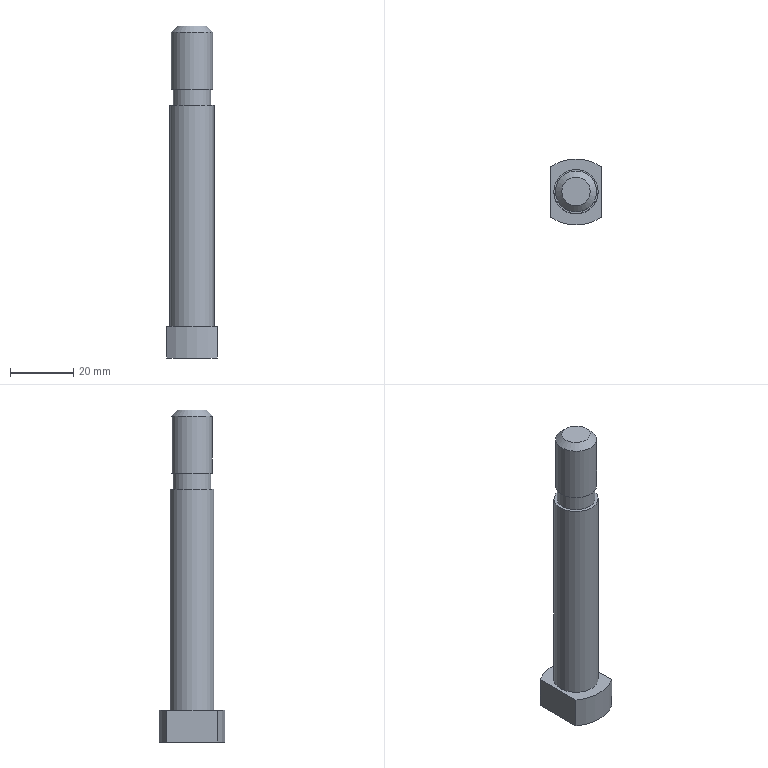Part | NX | features EXTRUDE 4, DATUM_CSYS 2, CHAMFER 1, SKETCH 1 | 1 solid | 13 faces | box 16 x 21.022 x 105 mm | volume 17029 mm3 | plane 7 | cylinder 5 | cone 1 | commonest cylinder face diameters 28 x2 12 x1 13 x1 14 x1
STEP:
#1=CARTESIAN_POINT('',(-8.,-8.,0.));
#2=VERTEX_POINT('',#1);
#3=CARTESIAN_POINT('',(-8.,8.,0.));
#4=VERTEX_POINT('',#3);
#5=CARTESIAN_POINT('',(-8.,-8.,0.));
#6=DIRECTION('',(0.,1.,0.));
#7=VECTOR('',#6,1000.);
#8=LINE('',#5,#7);
#9=EDGE_CURVE('',#2,#4,#8,.T.);
#10=ORIENTED_EDGE('',*,*,#9,.F.);
#11=CARTESIAN_POINT('',(-8.,-8.,10.));
#12=VERTEX_POINT('',#11);
#13=CARTESIAN_POINT('',(-8.,-8.,10.));
#14=DIRECTION('',(0.,0.,-1.));
#15=VECTOR('',#14,1000.);
#16=LINE('',#13,#15);
#17=EDGE_CURVE('',#12,#2,#16,.T.);
#18=ORIENTED_EDGE('',*,*,#17,.F.);
#19=CARTESIAN_POINT('',(-8.,8.,10.));
#20=VERTEX_POINT('',#19);
#21=CARTESIAN_POINT('',(-8.,-8.,10.));
#22=DIRECTION('',(0.,1.,0.));
#23=VECTOR('',#22,1000.);
#24=LINE('',#21,#23);
#25=EDGE_CURVE('',#12,#20,#24,.T.);
#26=ORIENTED_EDGE('',*,*,#25,.T.);
#27=CARTESIAN_POINT('',(-8.,8.,10.));
#28=DIRECTION('',(0.,0.,-1.));
#29=VECTOR('',#28,1000.);
#30=LINE('',#27,#29);
#31=EDGE_CURVE('',#20,#4,#30,.T.);
#32=ORIENTED_EDGE('',*,*,#31,.T.);
#33=EDGE_LOOP('',(#10,#18,#26,#32));
#34=FACE_BOUND('',#33,.T.);
#35=CARTESIAN_POINT('',(-8.,-8.,10.));
#36=DIRECTION('',(-1.,0.,0.));
#37=DIRECTION('',(0.,-1.,0.));
#38=AXIS2_PLACEMENT_3D('',#35,#36,#37);
#39=PLANE('',#38);
#40=ADVANCED_FACE('',(#34),#39,.T.);
#41=CARTESIAN_POINT('',(8.,8.,0.));
#42=VERTEX_POINT('',#41);
#43=CARTESIAN_POINT('',(0.,-3.489,0.));
#44=DIRECTION('',(0.,0.,-1.));
#45=DIRECTION('',(1.,0.,0.));
#46=AXIS2_PLACEMENT_3D('',#43,#44,#45);
#47=CIRCLE('',#46,14.);
#48=EDGE_CURVE('',#4,#42,#47,.T.);
#49=ORIENTED_EDGE('',*,*,#48,.F.);
#50=ORIENTED_EDGE('',*,*,#31,.F.);
#51=CARTESIAN_POINT('',(8.,8.,10.));
#52=VERTEX_POINT('',#51);
#53=CARTESIAN_POINT('',(0.,-3.489,10.));
#54=DIRECTION('',(0.,0.,-1.));
#55=DIRECTION('',(1.,0.,0.));
#56=AXIS2_PLACEMENT_3D('',#53,#54,#55);
#57=CIRCLE('',#56,14.);
#58=EDGE_CURVE('',#20,#52,#57,.T.);
#59=ORIENTED_EDGE('',*,*,#58,.T.);
#60=CARTESIAN_POINT('',(8.,8.,10.));
#61=DIRECTION('',(0.,0.,-1.));
#62=VECTOR('',#61,1000.);
#63=LINE('',#60,#62);
#64=EDGE_CURVE('',#52,#42,#63,.T.);
#65=ORIENTED_EDGE('',*,*,#64,.T.);
#66=EDGE_LOOP('',(#49,#50,#59,#65));
#67=FACE_BOUND('',#66,.T.);
#68=CARTESIAN_POINT('',(0.,-3.489,10.));
#69=DIRECTION('',(0.,0.,-1.));
#70=DIRECTION('',(-1.,0.,0.));
#71=AXIS2_PLACEMENT_3D('',#68,#69,#70);
#72=CYLINDRICAL_SURFACE('',#71,14.);
#73=ADVANCED_FACE('',(#67),#72,.T.);
#74=CARTESIAN_POINT('',(8.,-8.,0.));
#75=VERTEX_POINT('',#74);
#76=CARTESIAN_POINT('',(8.,8.,0.));
#77=DIRECTION('',(0.,-1.,0.));
#78=VECTOR('',#77,1000.);
#79=LINE('',#76,#78);
#80=EDGE_CURVE('',#42,#75,#79,.T.);
#81=ORIENTED_EDGE('',*,*,#80,.F.);
#82=ORIENTED_EDGE('',*,*,#64,.F.);
#83=CARTESIAN_POINT('',(8.,-8.,10.));
#84=VERTEX_POINT('',#83);
#85=CARTESIAN_POINT('',(8.,8.,10.));
#86=DIRECTION('',(0.,-1.,0.));
#87=VECTOR('',#86,1000.);
#88=LINE('',#85,#87);
#89=EDGE_CURVE('',#52,#84,#88,.T.);
#90=ORIENTED_EDGE('',*,*,#89,.T.);
#91=CARTESIAN_POINT('',(8.,-8.,10.));
#92=DIRECTION('',(0.,0.,-1.));
#93=VECTOR('',#92,1000.);
#94=LINE('',#91,#93);
#95=EDGE_CURVE('',#84,#75,#94,.T.);
#96=ORIENTED_EDGE('',*,*,#95,.T.);
#97=EDGE_LOOP('',(#81,#82,#90,#96));
#98=FACE_BOUND('',#97,.T.);
#99=CARTESIAN_POINT('',(8.,8.,10.));
#100=DIRECTION('',(1.,0.,0.));
#101=DIRECTION('',(0.,1.,0.));
#102=AXIS2_PLACEMENT_3D('',#99,#100,#101);
#103=PLANE('',#102);
#104=ADVANCED_FACE('',(#98),#103,.T.);
#105=CARTESIAN_POINT('',(0.,3.489,0.));
#106=DIRECTION('',(0.,0.,-1.));
#107=DIRECTION('',(1.,0.,0.));
#108=AXIS2_PLACEMENT_3D('',#105,#106,#107);
#109=CIRCLE('',#108,14.);
#110=EDGE_CURVE('',#75,#2,#109,.T.);
#111=ORIENTED_EDGE('',*,*,#110,.F.);
#112=ORIENTED_EDGE('',*,*,#95,.F.);
#113=CARTESIAN_POINT('',(0.,3.489,10.));
#114=DIRECTION('',(0.,0.,-1.));
#115=DIRECTION('',(1.,0.,0.));
#116=AXIS2_PLACEMENT_3D('',#113,#114,#115);
#117=CIRCLE('',#116,14.);
#118=EDGE_CURVE('',#84,#12,#117,.T.);
#119=ORIENTED_EDGE('',*,*,#118,.T.);
#120=ORIENTED_EDGE('',*,*,#17,.T.);
#121=EDGE_LOOP('',(#111,#112,#119,#120));
#122=FACE_BOUND('',#121,.T.);
#123=CARTESIAN_POINT('',(0.,3.489,10.));
#124=DIRECTION('',(0.,0.,-1.));
#125=DIRECTION('',(-1.,0.,0.));
#126=AXIS2_PLACEMENT_3D('',#123,#124,#125);
#127=CYLINDRICAL_SURFACE('',#126,14.);
#128=ADVANCED_FACE('',(#122),#127,.T.);
#129=CARTESIAN_POINT('',(7.,0.,10.));
#130=VERTEX_POINT('',#129);
#131=CARTESIAN_POINT('',(0.,0.,10.));
#132=DIRECTION('',(0.,0.,1.));
#133=DIRECTION('',(1.,0.,0.));
#134=AXIS2_PLACEMENT_3D('',#131,#132,#133);
#135=CIRCLE('',#134,7.);
#136=EDGE_CURVE('',#130,#130,#135,.T.);
#137=ORIENTED_EDGE('',*,*,#136,.F.);
#138=EDGE_LOOP('',(#137));
#139=FACE_BOUND('',#138,.T.);
#140=ORIENTED_EDGE('',*,*,#25,.F.);
#141=ORIENTED_EDGE('',*,*,#118,.F.);
#142=ORIENTED_EDGE('',*,*,#89,.F.);
#143=ORIENTED_EDGE('',*,*,#58,.F.);
#144=EDGE_LOOP('',(#140,#141,#142,#143));
#145=FACE_BOUND('',#144,.T.);
#146=CARTESIAN_POINT('',(0.,-3.489,10.));
#147=DIRECTION('',(0.,0.,-1.));
#148=DIRECTION('',(-1.,0.,0.));
#149=AXIS2_PLACEMENT_3D('',#146,#147,#148);
#150=PLANE('',#149);
#151=ADVANCED_FACE('',(#139,#145),#150,.F.);
#152=ORIENTED_EDGE('',*,*,#9,.T.);
#153=ORIENTED_EDGE('',*,*,#48,.T.);
#154=ORIENTED_EDGE('',*,*,#80,.T.);
#155=ORIENTED_EDGE('',*,*,#110,.T.);
#156=EDGE_LOOP('',(#152,#153,#154,#155));
#157=FACE_BOUND('',#156,.T.);
#158=CARTESIAN_POINT('',(0.,-3.489,0.));
#159=DIRECTION('',(0.,0.,-1.));
#160=DIRECTION('',(-1.,0.,0.));
#161=AXIS2_PLACEMENT_3D('',#158,#159,#160);
#162=PLANE('',#161);
#163=ADVANCED_FACE('',(#157),#162,.T.);
#164=CARTESIAN_POINT('',(7.,0.,80.));
#165=VERTEX_POINT('',#164);
#166=CARTESIAN_POINT('',(0.,0.,80.));
#167=DIRECTION('',(0.,0.,1.));
#168=DIRECTION('',(1.,0.,0.));
#169=AXIS2_PLACEMENT_3D('',#166,#167,#168);
#170=CIRCLE('',#169,7.);
#171=EDGE_CURVE('',#165,#165,#170,.T.);
#172=ORIENTED_EDGE('',*,*,#171,.F.);
#173=EDGE_LOOP('',(#172));
#174=FACE_BOUND('',#173,.T.);
#175=ORIENTED_EDGE('',*,*,#136,.T.);
#176=EDGE_LOOP('',(#175));
#177=FACE_BOUND('',#176,.T.);
#178=CARTESIAN_POINT('',(0.,0.,80.));
#179=DIRECTION('',(0.,0.,-1.));
#180=DIRECTION('',(-1.,0.,0.));
#181=AXIS2_PLACEMENT_3D('',#178,#179,#180);
#182=CYLINDRICAL_SURFACE('',#181,7.);
#183=ADVANCED_FACE('',(#174,#177),#182,.T.);
#184=CARTESIAN_POINT('',(6.,0.,80.));
#185=VERTEX_POINT('',#184);
#186=CARTESIAN_POINT('',(0.,0.,80.));
#187=DIRECTION('',(0.,0.,1.));
#188=DIRECTION('',(1.,0.,0.));
#189=AXIS2_PLACEMENT_3D('',#186,#187,#188);
#190=CIRCLE('',#189,6.);
#191=EDGE_CURVE('',#185,#185,#190,.T.);
#192=ORIENTED_EDGE('',*,*,#191,.F.);
#193=EDGE_LOOP('',(#192));
#194=FACE_BOUND('',#193,.T.);
#195=ORIENTED_EDGE('',*,*,#171,.T.);
#196=EDGE_LOOP('',(#195));
#197=FACE_BOUND('',#196,.T.);
#198=CARTESIAN_POINT('',(0.,0.,80.));
#199=DIRECTION('',(0.,0.,1.));
#200=DIRECTION('',(1.,0.,0.));
#201=AXIS2_PLACEMENT_3D('',#198,#199,#200);
#202=PLANE('',#201);
#203=ADVANCED_FACE('',(#194,#197),#202,.T.);
#204=CARTESIAN_POINT('',(6.,0.,85.));
#205=VERTEX_POINT('',#204);
#206=CARTESIAN_POINT('',(0.,0.,85.));
#207=DIRECTION('',(0.,0.,1.));
#208=DIRECTION('',(1.,0.,0.));
#209=AXIS2_PLACEMENT_3D('',#206,#207,#208);
#210=CIRCLE('',#209,6.);
#211=EDGE_CURVE('',#205,#205,#210,.T.);
#212=ORIENTED_EDGE('',*,*,#211,.F.);
#213=EDGE_LOOP('',(#212));
#214=FACE_BOUND('',#213,.T.);
#215=ORIENTED_EDGE('',*,*,#191,.T.);
#216=EDGE_LOOP('',(#215));
#217=FACE_BOUND('',#216,.T.);
#218=CARTESIAN_POINT('',(0.,0.,85.));
#219=DIRECTION('',(0.,0.,-1.));
#220=DIRECTION('',(-1.,0.,0.));
#221=AXIS2_PLACEMENT_3D('',#218,#219,#220);
#222=CYLINDRICAL_SURFACE('',#221,6.);
#223=ADVANCED_FACE('',(#214,#217),#222,.T.);
#224=CARTESIAN_POINT('',(6.5,0.,103.));
#225=VERTEX_POINT('',#224);
#226=CARTESIAN_POINT('',(0.,0.,103.));
#227=DIRECTION('',(0.,0.,1.));
#228=DIRECTION('',(1.,0.,0.));
#229=AXIS2_PLACEMENT_3D('',#226,#227,#228);
#230=CIRCLE('',#229,6.5);
#231=EDGE_CURVE('',#225,#225,#230,.F.);
#232=ORIENTED_EDGE('',*,*,#231,.T.);
#233=EDGE_LOOP('',(#232));
#234=FACE_BOUND('',#233,.T.);
#235=CARTESIAN_POINT('',(6.5,0.,85.));
#236=VERTEX_POINT('',#235);
#237=CARTESIAN_POINT('',(0.,0.,85.));
#238=DIRECTION('',(0.,0.,1.));
#239=DIRECTION('',(1.,0.,0.));
#240=AXIS2_PLACEMENT_3D('',#237,#238,#239);
#241=CIRCLE('',#240,6.5);
#242=EDGE_CURVE('',#236,#236,#241,.T.);
#243=ORIENTED_EDGE('',*,*,#242,.T.);
#244=EDGE_LOOP('',(#243));
#245=FACE_BOUND('',#244,.T.);
#246=CARTESIAN_POINT('',(0.,0.,105.));
#247=DIRECTION('',(0.,0.,-1.));
#248=DIRECTION('',(-1.,0.,0.));
#249=AXIS2_PLACEMENT_3D('',#246,#247,#248);
#250=CYLINDRICAL_SURFACE('',#249,6.5);
#251=ADVANCED_FACE('',(#234,#245),#250,.T.);
#252=CARTESIAN_POINT('',(4.5,0.,105.));
#253=VERTEX_POINT('',#252);
#254=CARTESIAN_POINT('',(0.,0.,105.));
#255=DIRECTION('',(0.,0.,1.));
#256=DIRECTION('',(1.,0.,0.));
#257=AXIS2_PLACEMENT_3D('',#254,#255,#256);
#258=CIRCLE('',#257,4.5);
#259=EDGE_CURVE('',#253,#253,#258,.T.);
#260=ORIENTED_EDGE('',*,*,#259,.T.);
#261=EDGE_LOOP('',(#260));
#262=FACE_BOUND('',#261,.T.);
#263=CARTESIAN_POINT('',(0.,0.,105.));
#264=DIRECTION('',(0.,0.,1.));
#265=DIRECTION('',(1.,0.,0.));
#266=AXIS2_PLACEMENT_3D('',#263,#264,#265);
#267=PLANE('',#266);
#268=ADVANCED_FACE('',(#262),#267,.T.);
#269=ORIENTED_EDGE('',*,*,#211,.T.);
#270=EDGE_LOOP('',(#269));
#271=FACE_BOUND('',#270,.T.);
#272=ORIENTED_EDGE('',*,*,#242,.F.);
#273=EDGE_LOOP('',(#272));
#274=FACE_BOUND('',#273,.T.);
#275=CARTESIAN_POINT('',(0.,0.,85.));
#276=DIRECTION('',(0.,0.,1.));
#277=DIRECTION('',(1.,0.,0.));
#278=AXIS2_PLACEMENT_3D('',#275,#276,#277);
#279=PLANE('',#278);
#280=ADVANCED_FACE('',(#271,#274),#279,.F.);
#281=ORIENTED_EDGE('',*,*,#231,.F.);
#282=EDGE_LOOP('',(#281));
#283=FACE_BOUND('',#282,.T.);
#284=ORIENTED_EDGE('',*,*,#259,.F.);
#285=EDGE_LOOP('',(#284));
#286=FACE_BOUND('',#285,.T.);
#287=CARTESIAN_POINT('',(0.,0.,105.));
#288=DIRECTION('',(0.,0.,-1.));
#289=DIRECTION('',(-1.,0.,0.));
#290=AXIS2_PLACEMENT_3D('',#287,#288,#289);
#291=CONICAL_SURFACE('',#290,4.5,0.7854);
#292=ADVANCED_FACE('',(#283,#286),#291,.T.);
#293=CLOSED_SHELL('',(#40,#73,#104,#128,#151,#163,#183,#203,#223,#251,#268,#280,#292));
#294=MANIFOLD_SOLID_BREP('',#293);
#295=(LENGTH_UNIT()NAMED_UNIT(*)SI_UNIT(.MILLI.,.METRE.));
#296=UNCERTAINTY_MEASURE_WITH_UNIT(LENGTH_MEASURE(0.00001),#295,'','');
#297=(NAMED_UNIT(*)PLANE_ANGLE_UNIT()SI_UNIT($,.RADIAN.));
#298=(NAMED_UNIT(*)SI_UNIT($,.STERADIAN.)SOLID_ANGLE_UNIT());
#299=(GEOMETRIC_REPRESENTATION_CONTEXT(3)GLOBAL_UNCERTAINTY_ASSIGNED_CONTEXT((#296))GLOBAL_UNIT_ASSIGNED_CONTEXT((#295,#297,#298))REPRESENTATION_CONTEXT('',''));
#300=ADVANCED_BREP_SHAPE_REPRESENTATION('',(#294),#299);